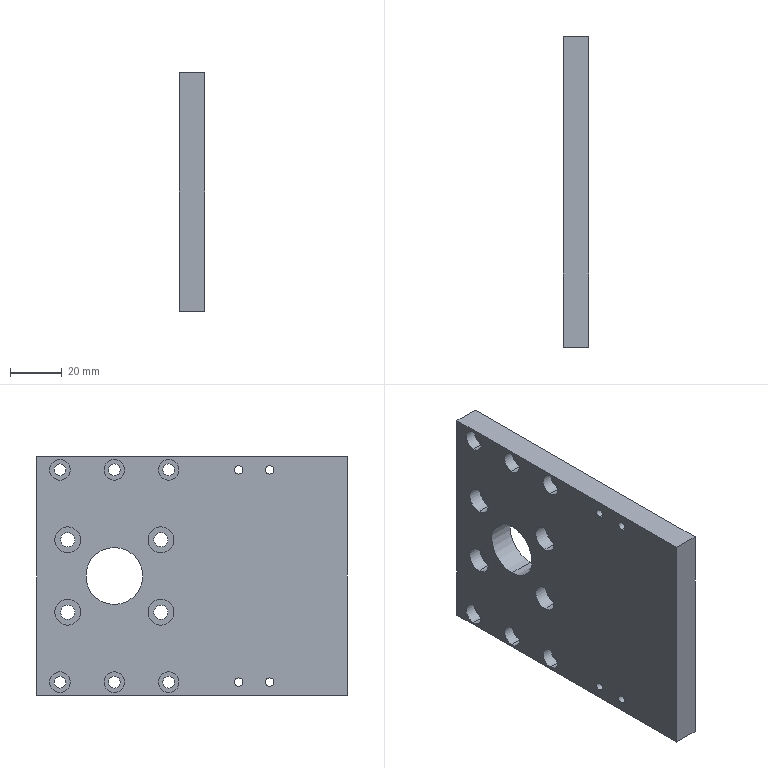Part | SolidWorks | features HoleWzd 3, Extrusion 1, ICE 1 | 1 solid | 66 faces | box 10 x 120 x 92 mm | volume 102262 mm3 | cylinder 50 | plane 16 | commonest cylinder face diameters 4.5 x12 8 x12 3.3 x8 5.5 x8 10 x8 22 x2